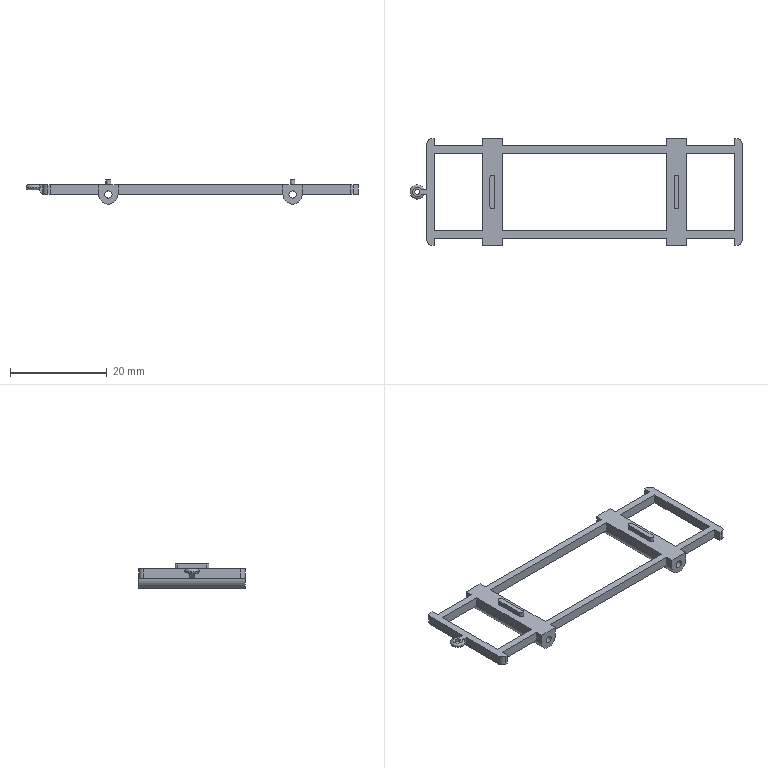Part | SolidWorks | features ICE 7, Extrusion 1, Fillet 1 | 1 solid | 75 faces | box 68.5 x 22 x 5 mm | volume 1025 mm3 | plane 56 | cylinder 16 | torus 3 | commonest cylinder face diameters 1 x6 1.5 x4 2 x4 4 x2